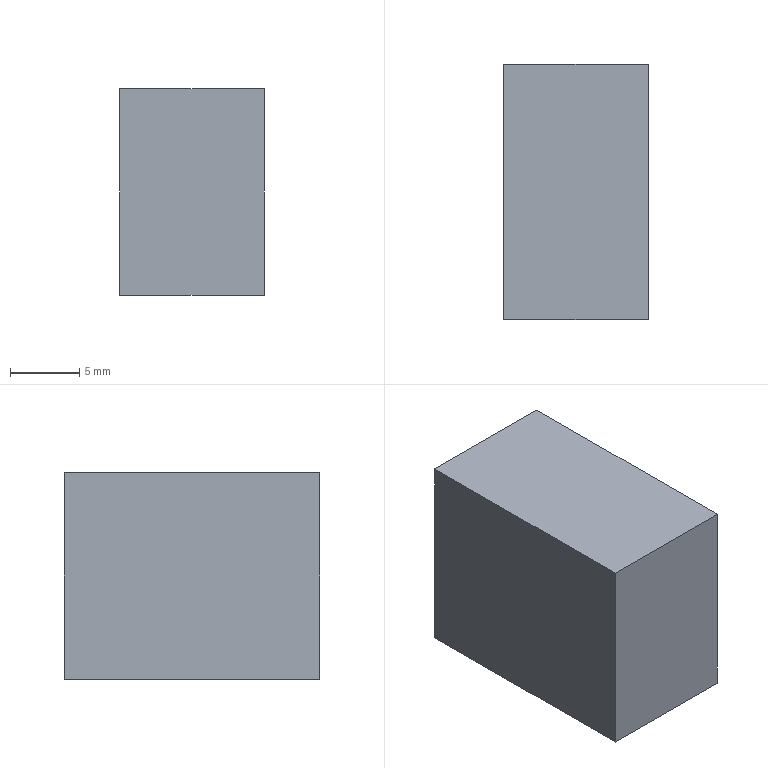Part | STEP file | RJ-USIO-V1_2-220411_19 | 1 solid | 6 faces | box 10.4 x 18.4 x 14.9 mm | volume 2851 mm3 | plane 6
STEP:
#1=CARTESIAN_POINT('',(0.,0.,0.));
#2=DIRECTION('',(0.,0.,1.));
#3=DIRECTION('',(1.,0.,0.));
#4=AXIS2_PLACEMENT_3D('',#1,#2,#3);
#5=CARTESIAN_POINT('',(43.7,13.8,15.3));
#6=VERTEX_POINT('',#5);
#7=CARTESIAN_POINT('',(43.7,32.2,15.3));
#8=VERTEX_POINT('',#7);
#9=CARTESIAN_POINT('',(43.7,13.8,15.3));
#10=DIRECTION('',(0.,1.,0.));
#11=VECTOR('',#10,1.);
#12=LINE('',#9,#11);
#13=CARTESIAN_POINT('',(43.7,13.8,15.3));
#14=DIRECTION('',(0.,0.,1.));
#15=DIRECTION('',(-1.,0.,0.));
#16=AXIS2_PLACEMENT_3D('',#13,#14,#15);
#17=PLANE('',#16);
#18=CARTESIAN_POINT('',(0.,0.));
#19=DIRECTION('',(0.,-1.));
#20=VECTOR('',#19,1.);
#21=LINE('',#18,#20);
#22=(GEOMETRIC_REPRESENTATION_CONTEXT(2)PARAMETRIC_REPRESENTATION_CONTEXT()REPRESENTATION_CONTEXT('',''));
#23=DEFINITIONAL_REPRESENTATION('',(#21),#22);
#24=PCURVE('',#17,#23);
#25=CARTESIAN_POINT('',(43.7,32.2,0.4));
#26=DIRECTION('',(1.,0.,0.));
#27=DIRECTION('',(0.,1.,0.));
#28=AXIS2_PLACEMENT_3D('',#25,#26,#27);
#29=PLANE('',#28);
#30=CARTESIAN_POINT('',(-18.4,14.9));
#31=DIRECTION('',(1.,0.));
#32=VECTOR('',#31,1.);
#33=LINE('',#30,#32);
#34=(GEOMETRIC_REPRESENTATION_CONTEXT(2)PARAMETRIC_REPRESENTATION_CONTEXT()REPRESENTATION_CONTEXT('',''));
#35=DEFINITIONAL_REPRESENTATION('',(#33),#34);
#36=PCURVE('',#29,#35);
#37=SURFACE_CURVE('',#12,(#24,#36),.PCURVE_S1.);
#38=EDGE_CURVE('',#6,#8,#37,.T.);
#39=ORIENTED_EDGE('',*,*,#38,.F.);
#40=CARTESIAN_POINT('',(33.3,13.8,15.3));
#41=VERTEX_POINT('',#40);
#42=CARTESIAN_POINT('',(33.3,13.8,15.3));
#43=DIRECTION('',(1.,0.,0.));
#44=VECTOR('',#43,1.);
#45=LINE('',#42,#44);
#46=CARTESIAN_POINT('',(10.4,0.));
#47=DIRECTION('',(-1.,0.));
#48=VECTOR('',#47,1.);
#49=LINE('',#46,#48);
#50=(GEOMETRIC_REPRESENTATION_CONTEXT(2)PARAMETRIC_REPRESENTATION_CONTEXT()REPRESENTATION_CONTEXT('',''));
#51=DEFINITIONAL_REPRESENTATION('',(#49),#50);
#52=PCURVE('',#17,#51);
#53=CARTESIAN_POINT('',(43.7,13.8,0.4));
#54=DIRECTION('',(0.,-1.,0.));
#55=DIRECTION('',(1.,0.,0.));
#56=AXIS2_PLACEMENT_3D('',#53,#54,#55);
#57=PLANE('',#56);
#58=CARTESIAN_POINT('',(-10.4,14.9));
#59=DIRECTION('',(1.,0.));
#60=VECTOR('',#59,1.);
#61=LINE('',#58,#60);
#62=(GEOMETRIC_REPRESENTATION_CONTEXT(2)PARAMETRIC_REPRESENTATION_CONTEXT()REPRESENTATION_CONTEXT('',''));
#63=DEFINITIONAL_REPRESENTATION('',(#61),#62);
#64=PCURVE('',#57,#63);
#65=SURFACE_CURVE('',#45,(#52,#64),.PCURVE_S1.);
#66=EDGE_CURVE('',#41,#6,#65,.T.);
#67=ORIENTED_EDGE('',*,*,#66,.F.);
#68=CARTESIAN_POINT('',(33.3,32.2,15.3));
#69=VERTEX_POINT('',#68);
#70=CARTESIAN_POINT('',(33.3,32.2,15.3));
#71=DIRECTION('',(0.,-1.,0.));
#72=VECTOR('',#71,1.);
#73=LINE('',#70,#72);
#74=CARTESIAN_POINT('',(10.4,-18.4));
#75=DIRECTION('',(0.,1.));
#76=VECTOR('',#75,1.);
#77=LINE('',#74,#76);
#78=(GEOMETRIC_REPRESENTATION_CONTEXT(2)PARAMETRIC_REPRESENTATION_CONTEXT()REPRESENTATION_CONTEXT('',''));
#79=DEFINITIONAL_REPRESENTATION('',(#77),#78);
#80=PCURVE('',#17,#79);
#81=CARTESIAN_POINT('',(33.3,13.8,0.4));
#82=DIRECTION('',(-1.,0.,0.));
#83=DIRECTION('',(0.,-1.,0.));
#84=AXIS2_PLACEMENT_3D('',#81,#82,#83);
#85=PLANE('',#84);
#86=CARTESIAN_POINT('',(-18.4,14.9));
#87=DIRECTION('',(1.,0.));
#88=VECTOR('',#87,1.);
#89=LINE('',#86,#88);
#90=(GEOMETRIC_REPRESENTATION_CONTEXT(2)PARAMETRIC_REPRESENTATION_CONTEXT()REPRESENTATION_CONTEXT('',''));
#91=DEFINITIONAL_REPRESENTATION('',(#89),#90);
#92=PCURVE('',#85,#91);
#93=SURFACE_CURVE('',#73,(#80,#92),.PCURVE_S1.);
#94=EDGE_CURVE('',#69,#41,#93,.T.);
#95=ORIENTED_EDGE('',*,*,#94,.F.);
#96=CARTESIAN_POINT('',(43.7,32.2,15.3));
#97=DIRECTION('',(-1.,0.,0.));
#98=VECTOR('',#97,1.);
#99=LINE('',#96,#98);
#100=CARTESIAN_POINT('',(0.,-18.4));
#101=DIRECTION('',(1.,0.));
#102=VECTOR('',#101,1.);
#103=LINE('',#100,#102);
#104=(GEOMETRIC_REPRESENTATION_CONTEXT(2)PARAMETRIC_REPRESENTATION_CONTEXT()REPRESENTATION_CONTEXT('',''));
#105=DEFINITIONAL_REPRESENTATION('',(#103),#104);
#106=PCURVE('',#17,#105);
#107=CARTESIAN_POINT('',(33.3,32.2,0.4));
#108=DIRECTION('',(0.,1.,0.));
#109=DIRECTION('',(-1.,0.,0.));
#110=AXIS2_PLACEMENT_3D('',#107,#108,#109);
#111=PLANE('',#110);
#112=CARTESIAN_POINT('',(-10.4,14.9));
#113=DIRECTION('',(1.,0.));
#114=VECTOR('',#113,1.);
#115=LINE('',#112,#114);
#116=(GEOMETRIC_REPRESENTATION_CONTEXT(2)PARAMETRIC_REPRESENTATION_CONTEXT()REPRESENTATION_CONTEXT('',''));
#117=DEFINITIONAL_REPRESENTATION('',(#115),#116);
#118=PCURVE('',#111,#117);
#119=SURFACE_CURVE('',#99,(#106,#118),.PCURVE_S1.);
#120=EDGE_CURVE('',#8,#69,#119,.T.);
#121=ORIENTED_EDGE('',*,*,#120,.F.);
#122=EDGE_LOOP('',(#39,#67,#95,#121));
#123=FACE_BOUND('',#122,.F.);
#124=ADVANCED_FACE('',(#123),#17,.T.);
#125=CARTESIAN_POINT('',(43.7,32.2,0.4));
#126=VERTEX_POINT('',#125);
#127=CARTESIAN_POINT('',(43.7,32.2,15.3));
#128=DIRECTION('',(0.,0.,-1.));
#129=VECTOR('',#128,1.);
#130=LINE('',#127,#129);
#131=CARTESIAN_POINT('',(0.,14.9));
#132=DIRECTION('',(0.,-1.));
#133=VECTOR('',#132,1.);
#134=LINE('',#131,#133);
#135=(GEOMETRIC_REPRESENTATION_CONTEXT(2)PARAMETRIC_REPRESENTATION_CONTEXT()REPRESENTATION_CONTEXT('',''));
#136=DEFINITIONAL_REPRESENTATION('',(#134),#135);
#137=PCURVE('',#29,#136);
#138=CARTESIAN_POINT('',(-10.4,14.9));
#139=DIRECTION('',(0.,-1.));
#140=VECTOR('',#139,1.);
#141=LINE('',#138,#140);
#142=(GEOMETRIC_REPRESENTATION_CONTEXT(2)PARAMETRIC_REPRESENTATION_CONTEXT()REPRESENTATION_CONTEXT('',''));
#143=DEFINITIONAL_REPRESENTATION('',(#141),#142);
#144=PCURVE('',#111,#143);
#145=SURFACE_CURVE('',#130,(#137,#144),.PCURVE_S1.);
#146=EDGE_CURVE('',#8,#126,#145,.T.);
#147=ORIENTED_EDGE('',*,*,#146,.T.);
#148=CARTESIAN_POINT('',(43.7,13.8,0.4));
#149=VERTEX_POINT('',#148);
#150=CARTESIAN_POINT('',(43.7,13.8,0.4));
#151=DIRECTION('',(0.,1.,0.));
#152=VECTOR('',#151,1.);
#153=LINE('',#150,#152);
#154=CARTESIAN_POINT('',(-18.4,0.));
#155=DIRECTION('',(1.,0.));
#156=VECTOR('',#155,1.);
#157=LINE('',#154,#156);
#158=(GEOMETRIC_REPRESENTATION_CONTEXT(2)PARAMETRIC_REPRESENTATION_CONTEXT()REPRESENTATION_CONTEXT('',''));
#159=DEFINITIONAL_REPRESENTATION('',(#157),#158);
#160=PCURVE('',#29,#159);
#161=CARTESIAN_POINT('',(43.7,13.8,0.4));
#162=DIRECTION('',(0.,0.,1.));
#163=DIRECTION('',(-1.,0.,0.));
#164=AXIS2_PLACEMENT_3D('',#161,#162,#163);
#165=PLANE('',#164);
#166=CARTESIAN_POINT('',(0.,0.));
#167=DIRECTION('',(0.,-1.));
#168=VECTOR('',#167,1.);
#169=LINE('',#166,#168);
#170=(GEOMETRIC_REPRESENTATION_CONTEXT(2)PARAMETRIC_REPRESENTATION_CONTEXT()REPRESENTATION_CONTEXT('',''));
#171=DEFINITIONAL_REPRESENTATION('',(#169),#170);
#172=PCURVE('',#165,#171);
#173=SURFACE_CURVE('',#153,(#160,#172),.PCURVE_S1.);
#174=EDGE_CURVE('',#149,#126,#173,.T.);
#175=ORIENTED_EDGE('',*,*,#174,.F.);
#176=CARTESIAN_POINT('',(43.7,13.8,15.3));
#177=DIRECTION('',(0.,0.,-1.));
#178=VECTOR('',#177,1.);
#179=LINE('',#176,#178);
#180=CARTESIAN_POINT('',(-18.4,14.9));
#181=DIRECTION('',(0.,-1.));
#182=VECTOR('',#181,1.);
#183=LINE('',#180,#182);
#184=(GEOMETRIC_REPRESENTATION_CONTEXT(2)PARAMETRIC_REPRESENTATION_CONTEXT()REPRESENTATION_CONTEXT('',''));
#185=DEFINITIONAL_REPRESENTATION('',(#183),#184);
#186=PCURVE('',#29,#185);
#187=CARTESIAN_POINT('',(0.,14.9));
#188=DIRECTION('',(0.,-1.));
#189=VECTOR('',#188,1.);
#190=LINE('',#187,#189);
#191=(GEOMETRIC_REPRESENTATION_CONTEXT(2)PARAMETRIC_REPRESENTATION_CONTEXT()REPRESENTATION_CONTEXT('',''));
#192=DEFINITIONAL_REPRESENTATION('',(#190),#191);
#193=PCURVE('',#57,#192);
#194=SURFACE_CURVE('',#179,(#186,#193),.PCURVE_S1.);
#195=EDGE_CURVE('',#6,#149,#194,.T.);
#196=ORIENTED_EDGE('',*,*,#195,.F.);
#197=ORIENTED_EDGE('',*,*,#38,.T.);
#198=EDGE_LOOP('',(#147,#175,#196,#197));
#199=FACE_BOUND('',#198,.F.);
#200=ADVANCED_FACE('',(#199),#29,.T.);
#201=CARTESIAN_POINT('',(33.3,32.2,0.4));
#202=VERTEX_POINT('',#201);
#203=CARTESIAN_POINT('',(33.3,32.2,15.3));
#204=DIRECTION('',(0.,0.,-1.));
#205=VECTOR('',#204,1.);
#206=LINE('',#203,#205);
#207=CARTESIAN_POINT('',(0.,14.9));
#208=DIRECTION('',(0.,-1.));
#209=VECTOR('',#208,1.);
#210=LINE('',#207,#209);
#211=(GEOMETRIC_REPRESENTATION_CONTEXT(2)PARAMETRIC_REPRESENTATION_CONTEXT()REPRESENTATION_CONTEXT('',''));
#212=DEFINITIONAL_REPRESENTATION('',(#210),#211);
#213=PCURVE('',#111,#212);
#214=CARTESIAN_POINT('',(-18.4,14.9));
#215=DIRECTION('',(0.,-1.));
#216=VECTOR('',#215,1.);
#217=LINE('',#214,#216);
#218=(GEOMETRIC_REPRESENTATION_CONTEXT(2)PARAMETRIC_REPRESENTATION_CONTEXT()REPRESENTATION_CONTEXT('',''));
#219=DEFINITIONAL_REPRESENTATION('',(#217),#218);
#220=PCURVE('',#85,#219);
#221=SURFACE_CURVE('',#206,(#213,#220),.PCURVE_S1.);
#222=EDGE_CURVE('',#69,#202,#221,.T.);
#223=ORIENTED_EDGE('',*,*,#222,.T.);
#224=CARTESIAN_POINT('',(43.7,32.2,0.4));
#225=DIRECTION('',(-1.,0.,0.));
#226=VECTOR('',#225,1.);
#227=LINE('',#224,#226);
#228=CARTESIAN_POINT('',(-10.4,0.));
#229=DIRECTION('',(1.,0.));
#230=VECTOR('',#229,1.);
#231=LINE('',#228,#230);
#232=(GEOMETRIC_REPRESENTATION_CONTEXT(2)PARAMETRIC_REPRESENTATION_CONTEXT()REPRESENTATION_CONTEXT('',''));
#233=DEFINITIONAL_REPRESENTATION('',(#231),#232);
#234=PCURVE('',#111,#233);
#235=CARTESIAN_POINT('',(0.,-18.4));
#236=DIRECTION('',(1.,0.));
#237=VECTOR('',#236,1.);
#238=LINE('',#235,#237);
#239=(GEOMETRIC_REPRESENTATION_CONTEXT(2)PARAMETRIC_REPRESENTATION_CONTEXT()REPRESENTATION_CONTEXT('',''));
#240=DEFINITIONAL_REPRESENTATION('',(#238),#239);
#241=PCURVE('',#165,#240);
#242=SURFACE_CURVE('',#227,(#234,#241),.PCURVE_S1.);
#243=EDGE_CURVE('',#126,#202,#242,.T.);
#244=ORIENTED_EDGE('',*,*,#243,.F.);
#245=ORIENTED_EDGE('',*,*,#146,.F.);
#246=ORIENTED_EDGE('',*,*,#120,.T.);
#247=EDGE_LOOP('',(#223,#244,#245,#246));
#248=FACE_BOUND('',#247,.F.);
#249=ADVANCED_FACE('',(#248),#111,.T.);
#250=CARTESIAN_POINT('',(33.3,13.8,0.4));
#251=VERTEX_POINT('',#250);
#252=CARTESIAN_POINT('',(33.3,13.8,15.3));
#253=DIRECTION('',(0.,0.,-1.));
#254=VECTOR('',#253,1.);
#255=LINE('',#252,#254);
#256=CARTESIAN_POINT('',(0.,14.9));
#257=DIRECTION('',(0.,-1.));
#258=VECTOR('',#257,1.);
#259=LINE('',#256,#258);
#260=(GEOMETRIC_REPRESENTATION_CONTEXT(2)PARAMETRIC_REPRESENTATION_CONTEXT()REPRESENTATION_CONTEXT('',''));
#261=DEFINITIONAL_REPRESENTATION('',(#259),#260);
#262=PCURVE('',#85,#261);
#263=CARTESIAN_POINT('',(-10.4,14.9));
#264=DIRECTION('',(0.,-1.));
#265=VECTOR('',#264,1.);
#266=LINE('',#263,#265);
#267=(GEOMETRIC_REPRESENTATION_CONTEXT(2)PARAMETRIC_REPRESENTATION_CONTEXT()REPRESENTATION_CONTEXT('',''));
#268=DEFINITIONAL_REPRESENTATION('',(#266),#267);
#269=PCURVE('',#57,#268);
#270=SURFACE_CURVE('',#255,(#262,#269),.PCURVE_S1.);
#271=EDGE_CURVE('',#41,#251,#270,.T.);
#272=ORIENTED_EDGE('',*,*,#271,.T.);
#273=CARTESIAN_POINT('',(33.3,32.2,0.4));
#274=DIRECTION('',(0.,-1.,0.));
#275=VECTOR('',#274,1.);
#276=LINE('',#273,#275);
#277=CARTESIAN_POINT('',(-18.4,0.));
#278=DIRECTION('',(1.,0.));
#279=VECTOR('',#278,1.);
#280=LINE('',#277,#279);
#281=(GEOMETRIC_REPRESENTATION_CONTEXT(2)PARAMETRIC_REPRESENTATION_CONTEXT()REPRESENTATION_CONTEXT('',''));
#282=DEFINITIONAL_REPRESENTATION('',(#280),#281);
#283=PCURVE('',#85,#282);
#284=CARTESIAN_POINT('',(10.4,-18.4));
#285=DIRECTION('',(0.,1.));
#286=VECTOR('',#285,1.);
#287=LINE('',#284,#286);
#288=(GEOMETRIC_REPRESENTATION_CONTEXT(2)PARAMETRIC_REPRESENTATION_CONTEXT()REPRESENTATION_CONTEXT('',''));
#289=DEFINITIONAL_REPRESENTATION('',(#287),#288);
#290=PCURVE('',#165,#289);
#291=SURFACE_CURVE('',#276,(#283,#290),.PCURVE_S1.);
#292=EDGE_CURVE('',#202,#251,#291,.T.);
#293=ORIENTED_EDGE('',*,*,#292,.F.);
#294=ORIENTED_EDGE('',*,*,#222,.F.);
#295=ORIENTED_EDGE('',*,*,#94,.T.);
#296=EDGE_LOOP('',(#272,#293,#294,#295));
#297=FACE_BOUND('',#296,.F.);
#298=ADVANCED_FACE('',(#297),#85,.T.);
#299=ORIENTED_EDGE('',*,*,#195,.T.);
#300=CARTESIAN_POINT('',(33.3,13.8,0.4));
#301=DIRECTION('',(1.,0.,0.));
#302=VECTOR('',#301,1.);
#303=LINE('',#300,#302);
#304=CARTESIAN_POINT('',(-10.4,0.));
#305=DIRECTION('',(1.,0.));
#306=VECTOR('',#305,1.);
#307=LINE('',#304,#306);
#308=(GEOMETRIC_REPRESENTATION_CONTEXT(2)PARAMETRIC_REPRESENTATION_CONTEXT()REPRESENTATION_CONTEXT('',''));
#309=DEFINITIONAL_REPRESENTATION('',(#307),#308);
#310=PCURVE('',#57,#309);
#311=CARTESIAN_POINT('',(10.4,0.));
#312=DIRECTION('',(-1.,0.));
#313=VECTOR('',#312,1.);
#314=LINE('',#311,#313);
#315=(GEOMETRIC_REPRESENTATION_CONTEXT(2)PARAMETRIC_REPRESENTATION_CONTEXT()REPRESENTATION_CONTEXT('',''));
#316=DEFINITIONAL_REPRESENTATION('',(#314),#315);
#317=PCURVE('',#165,#316);
#318=SURFACE_CURVE('',#303,(#310,#317),.PCURVE_S1.);
#319=EDGE_CURVE('',#251,#149,#318,.T.);
#320=ORIENTED_EDGE('',*,*,#319,.F.);
#321=ORIENTED_EDGE('',*,*,#271,.F.);
#322=ORIENTED_EDGE('',*,*,#66,.T.);
#323=EDGE_LOOP('',(#299,#320,#321,#322));
#324=FACE_BOUND('',#323,.F.);
#325=ADVANCED_FACE('',(#324),#57,.T.);
#326=ORIENTED_EDGE('',*,*,#319,.T.);
#327=ORIENTED_EDGE('',*,*,#174,.T.);
#328=ORIENTED_EDGE('',*,*,#243,.T.);
#329=ORIENTED_EDGE('',*,*,#292,.T.);
#330=EDGE_LOOP('',(#326,#327,#328,#329));
#331=FACE_BOUND('',#330,.F.);
#332=ADVANCED_FACE('',(#331),#165,.F.);
#333=CLOSED_SHELL('',(#124,#200,#249,#298,#325,#332));
#334=MANIFOLD_SOLID_BREP('',#333);
#335=(LENGTH_UNIT()NAMED_UNIT(*)SI_UNIT(.MILLI.,.METRE.));
#336=UNCERTAINTY_MEASURE_WITH_UNIT(LENGTH_MEASURE(0.0000001),#335,'','');
#337=(NAMED_UNIT(*)PLANE_ANGLE_UNIT()SI_UNIT($,.RADIAN.));
#338=(NAMED_UNIT(*)SI_UNIT($,.STERADIAN.)SOLID_ANGLE_UNIT());
#339=(GEOMETRIC_REPRESENTATION_CONTEXT(3)GLOBAL_UNCERTAINTY_ASSIGNED_CONTEXT((#336))GLOBAL_UNIT_ASSIGNED_CONTEXT((#335,#337,#338))REPRESENTATION_CONTEXT('',''));
#340=ADVANCED_BREP_SHAPE_REPRESENTATION('',(#4,#334),#339);